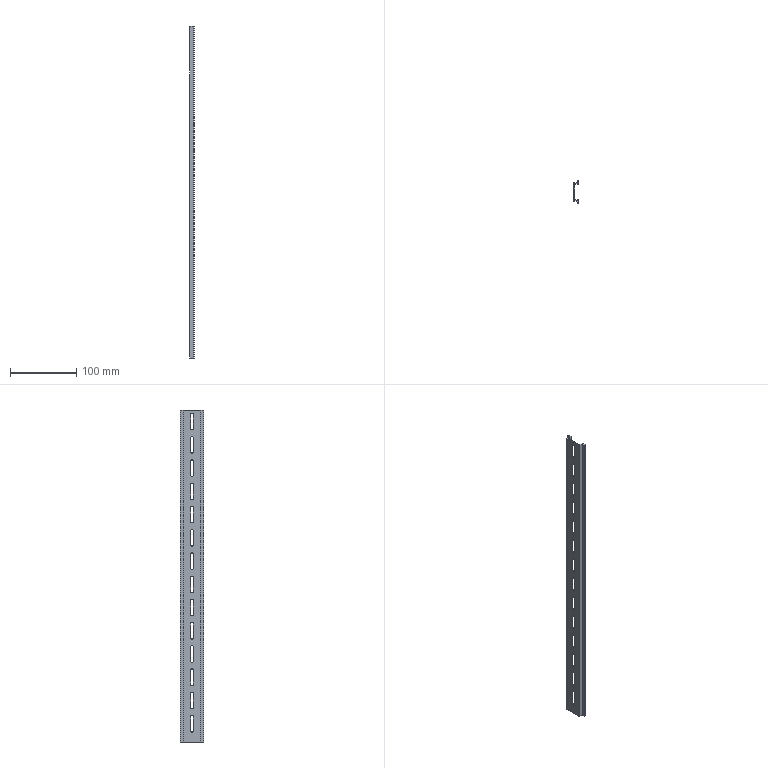Part | STEP file | [SDR-1(500)] | 1 solid | 70 faces | box 7.5 x 35 x 500 mm | volume 32979 mm3 | plane 42 | cylinder 28 | commonest cylinder face diameters 4.5 x28